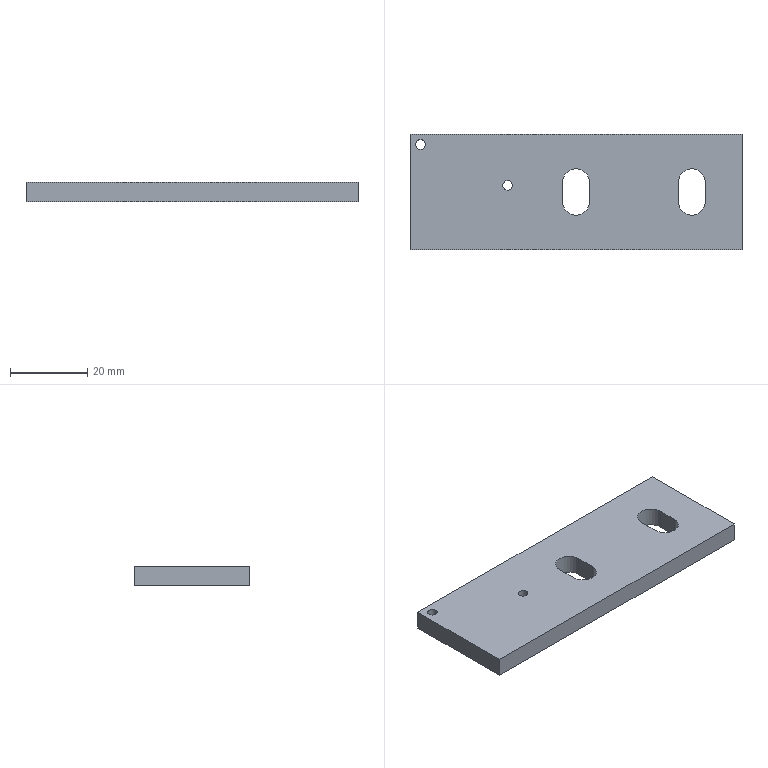Part | STEP file | Square proximity switch plate | 1 solid | 18 faces | box 86 x 30 x 5 mm | volume 12116 mm3 | plane 10 | cylinder 8 | commonest cylinder face diameters 2.5 x4 7 x4
STEP:
#1=CARTESIAN_POINT('',(0.,0.,0.));
#2=DIRECTION('',(0.,0.,1.));
#3=DIRECTION('',(1.,0.,0.));
#4=AXIS2_PLACEMENT_3D('',#1,#2,#3);
#5=CARTESIAN_POINT('',(-16.45,1.7,0.));
#6=VERTEX_POINT('',#5);
#7=CARTESIAN_POINT('',(-16.45,1.7,5.));
#8=VERTEX_POINT('',#7);
#9=CARTESIAN_POINT('',(-16.45,1.7,5.));
#10=DIRECTION('',(0.,0.,1.));
#11=VECTOR('',#10,1.);
#12=LINE('',#9,#11);
#13=CARTESIAN_POINT('',(-17.7,1.7,5.));
#14=DIRECTION('',(0.,0.,1.));
#15=DIRECTION('',(1.,0.,0.));
#16=AXIS2_PLACEMENT_3D('',#13,#14,#15);
#17=CYLINDRICAL_SURFACE('',#16,1.25);
#18=CARTESIAN_POINT('',(6.283,0.));
#19=DIRECTION('',(0.,1.));
#20=VECTOR('',#19,1.);
#21=LINE('',#18,#20);
#22=(GEOMETRIC_REPRESENTATION_CONTEXT(2)PARAMETRIC_REPRESENTATION_CONTEXT()REPRESENTATION_CONTEXT('',''));
#23=DEFINITIONAL_REPRESENTATION('',(#21),#22);
#24=PCURVE('',#17,#23);
#25=CARTESIAN_POINT('',(-17.7,1.7,5.));
#26=DIRECTION('',(0.,0.,1.));
#27=DIRECTION('',(1.,0.,0.));
#28=AXIS2_PLACEMENT_3D('',#25,#26,#27);
#29=CYLINDRICAL_SURFACE('',#28,1.25);
#30=CARTESIAN_POINT('',(0.,0.));
#31=DIRECTION('',(0.,1.));
#32=VECTOR('',#31,1.);
#33=LINE('',#30,#32);
#34=(GEOMETRIC_REPRESENTATION_CONTEXT(2)PARAMETRIC_REPRESENTATION_CONTEXT()REPRESENTATION_CONTEXT('',''));
#35=DEFINITIONAL_REPRESENTATION('',(#33),#34);
#36=PCURVE('',#29,#35);
#37=SURFACE_CURVE('',#12,(#24,#36),.PCURVE_S1.);
#38=EDGE_CURVE('',#6,#8,#37,.T.);
#39=ORIENTED_EDGE('',*,*,#38,.T.);
#40=CARTESIAN_POINT('',(-18.95,1.7,5.));
#41=VERTEX_POINT('',#40);
#42=CARTESIAN_POINT('',(-17.7,1.7,5.));
#43=DIRECTION('',(0.,0.,1.));
#44=DIRECTION('',(1.,0.,0.));
#45=AXIS2_PLACEMENT_3D('',#42,#43,#44);
#46=CIRCLE('',#45,1.25);
#47=CARTESIAN_POINT('',(0.,0.));
#48=DIRECTION('',(1.,0.));
#49=VECTOR('',#48,1.);
#50=LINE('',#47,#49);
#51=(GEOMETRIC_REPRESENTATION_CONTEXT(2)PARAMETRIC_REPRESENTATION_CONTEXT()REPRESENTATION_CONTEXT('',''));
#52=DEFINITIONAL_REPRESENTATION('',(#50),#51);
#53=PCURVE('',#17,#52);
#54=CARTESIAN_POINT('',(0.,0.,5.));
#55=DIRECTION('',(0.,0.,1.));
#56=DIRECTION('',(1.,0.,0.));
#57=AXIS2_PLACEMENT_3D('',#54,#55,#56);
#58=PLANE('',#57);
#59=CARTESIAN_POINT('',(-17.7,1.7));
#60=DIRECTION('',(1.,0.));
#61=AXIS2_PLACEMENT_2D('',#59,#60);
#62=CIRCLE('',#61,1.25);
#63=(GEOMETRIC_REPRESENTATION_CONTEXT(2)PARAMETRIC_REPRESENTATION_CONTEXT()REPRESENTATION_CONTEXT('',''));
#64=DEFINITIONAL_REPRESENTATION('',(#62),#63);
#65=PCURVE('',#58,#64);
#66=SURFACE_CURVE('',#46,(#53,#65),.PCURVE_S1.);
#67=EDGE_CURVE('',#41,#8,#66,.T.);
#68=ORIENTED_EDGE('',*,*,#67,.F.);
#69=CARTESIAN_POINT('',(-18.95,1.7,0.));
#70=VERTEX_POINT('',#69);
#71=CARTESIAN_POINT('',(-18.95,1.7,5.));
#72=DIRECTION('',(0.,0.,1.));
#73=VECTOR('',#72,1.);
#74=LINE('',#71,#73);
#75=CARTESIAN_POINT('',(3.142,0.));
#76=DIRECTION('',(0.,1.));
#77=VECTOR('',#76,1.);
#78=LINE('',#75,#77);
#79=(GEOMETRIC_REPRESENTATION_CONTEXT(2)PARAMETRIC_REPRESENTATION_CONTEXT()REPRESENTATION_CONTEXT('',''));
#80=DEFINITIONAL_REPRESENTATION('',(#78),#79);
#81=PCURVE('',#17,#80);
#82=CARTESIAN_POINT('',(3.142,0.));
#83=DIRECTION('',(0.,1.));
#84=VECTOR('',#83,1.);
#85=LINE('',#82,#84);
#86=(GEOMETRIC_REPRESENTATION_CONTEXT(2)PARAMETRIC_REPRESENTATION_CONTEXT()REPRESENTATION_CONTEXT('',''));
#87=DEFINITIONAL_REPRESENTATION('',(#85),#86);
#88=PCURVE('',#29,#87);
#89=SURFACE_CURVE('',#74,(#81,#88),.PCURVE_S1.);
#90=EDGE_CURVE('',#70,#41,#89,.T.);
#91=ORIENTED_EDGE('',*,*,#90,.F.);
#92=CARTESIAN_POINT('',(-17.7,1.7,0.));
#93=DIRECTION('',(0.,0.,1.));
#94=DIRECTION('',(1.,0.,0.));
#95=AXIS2_PLACEMENT_3D('',#92,#93,#94);
#96=CIRCLE('',#95,1.25);
#97=CARTESIAN_POINT('',(0.,-5.));
#98=DIRECTION('',(1.,0.));
#99=VECTOR('',#98,1.);
#100=LINE('',#97,#99);
#101=(GEOMETRIC_REPRESENTATION_CONTEXT(2)PARAMETRIC_REPRESENTATION_CONTEXT()REPRESENTATION_CONTEXT('',''));
#102=DEFINITIONAL_REPRESENTATION('',(#100),#101);
#103=PCURVE('',#17,#102);
#104=CARTESIAN_POINT('',(0.,0.,0.));
#105=DIRECTION('',(0.,0.,1.));
#106=DIRECTION('',(1.,0.,0.));
#107=AXIS2_PLACEMENT_3D('',#104,#105,#106);
#108=PLANE('',#107);
#109=CARTESIAN_POINT('',(-17.7,1.7));
#110=DIRECTION('',(1.,0.));
#111=AXIS2_PLACEMENT_2D('',#109,#110);
#112=CIRCLE('',#111,1.25);
#113=(GEOMETRIC_REPRESENTATION_CONTEXT(2)PARAMETRIC_REPRESENTATION_CONTEXT()REPRESENTATION_CONTEXT('',''));
#114=DEFINITIONAL_REPRESENTATION('',(#112),#113);
#115=PCURVE('',#108,#114);
#116=SURFACE_CURVE('',#96,(#103,#115),.PCURVE_S1.);
#117=EDGE_CURVE('',#70,#6,#116,.T.);
#118=ORIENTED_EDGE('',*,*,#117,.T.);
#119=EDGE_LOOP('',(#39,#68,#91,#118));
#120=FACE_BOUND('',#119,.F.);
#121=ADVANCED_FACE('',(#120),#17,.F.);
#122=CARTESIAN_POINT('',(-39.05,12.3,0.));
#123=VERTEX_POINT('',#122);
#124=CARTESIAN_POINT('',(-39.05,12.3,5.));
#125=VERTEX_POINT('',#124);
#126=CARTESIAN_POINT('',(-39.05,12.3,5.));
#127=DIRECTION('',(0.,0.,1.));
#128=VECTOR('',#127,1.);
#129=LINE('',#126,#128);
#130=CARTESIAN_POINT('',(-40.3,12.3,5.));
#131=DIRECTION('',(0.,0.,1.));
#132=DIRECTION('',(1.,0.,0.));
#133=AXIS2_PLACEMENT_3D('',#130,#131,#132);
#134=CYLINDRICAL_SURFACE('',#133,1.25);
#135=CARTESIAN_POINT('',(6.283,0.));
#136=DIRECTION('',(0.,1.));
#137=VECTOR('',#136,1.);
#138=LINE('',#135,#137);
#139=(GEOMETRIC_REPRESENTATION_CONTEXT(2)PARAMETRIC_REPRESENTATION_CONTEXT()REPRESENTATION_CONTEXT('',''));
#140=DEFINITIONAL_REPRESENTATION('',(#138),#139);
#141=PCURVE('',#134,#140);
#142=CARTESIAN_POINT('',(-40.3,12.3,5.));
#143=DIRECTION('',(0.,0.,1.));
#144=DIRECTION('',(1.,0.,0.));
#145=AXIS2_PLACEMENT_3D('',#142,#143,#144);
#146=CYLINDRICAL_SURFACE('',#145,1.25);
#147=CARTESIAN_POINT('',(0.,0.));
#148=DIRECTION('',(0.,1.));
#149=VECTOR('',#148,1.);
#150=LINE('',#147,#149);
#151=(GEOMETRIC_REPRESENTATION_CONTEXT(2)PARAMETRIC_REPRESENTATION_CONTEXT()REPRESENTATION_CONTEXT('',''));
#152=DEFINITIONAL_REPRESENTATION('',(#150),#151);
#153=PCURVE('',#146,#152);
#154=SURFACE_CURVE('',#129,(#141,#153),.PCURVE_S1.);
#155=EDGE_CURVE('',#123,#125,#154,.T.);
#156=ORIENTED_EDGE('',*,*,#155,.T.);
#157=CARTESIAN_POINT('',(-41.55,12.3,5.));
#158=VERTEX_POINT('',#157);
#159=CARTESIAN_POINT('',(-40.3,12.3,5.));
#160=DIRECTION('',(0.,0.,1.));
#161=DIRECTION('',(1.,0.,0.));
#162=AXIS2_PLACEMENT_3D('',#159,#160,#161);
#163=CIRCLE('',#162,1.25);
#164=CARTESIAN_POINT('',(0.,0.));
#165=DIRECTION('',(1.,0.));
#166=VECTOR('',#165,1.);
#167=LINE('',#164,#166);
#168=(GEOMETRIC_REPRESENTATION_CONTEXT(2)PARAMETRIC_REPRESENTATION_CONTEXT()REPRESENTATION_CONTEXT('',''));
#169=DEFINITIONAL_REPRESENTATION('',(#167),#168);
#170=PCURVE('',#134,#169);
#171=CARTESIAN_POINT('',(-40.3,12.3));
#172=DIRECTION('',(1.,0.));
#173=AXIS2_PLACEMENT_2D('',#171,#172);
#174=CIRCLE('',#173,1.25);
#175=(GEOMETRIC_REPRESENTATION_CONTEXT(2)PARAMETRIC_REPRESENTATION_CONTEXT()REPRESENTATION_CONTEXT('',''));
#176=DEFINITIONAL_REPRESENTATION('',(#174),#175);
#177=PCURVE('',#58,#176);
#178=SURFACE_CURVE('',#163,(#170,#177),.PCURVE_S1.);
#179=EDGE_CURVE('',#158,#125,#178,.T.);
#180=ORIENTED_EDGE('',*,*,#179,.F.);
#181=CARTESIAN_POINT('',(-41.55,12.3,0.));
#182=VERTEX_POINT('',#181);
#183=CARTESIAN_POINT('',(-41.55,12.3,5.));
#184=DIRECTION('',(0.,0.,1.));
#185=VECTOR('',#184,1.);
#186=LINE('',#183,#185);
#187=CARTESIAN_POINT('',(3.142,0.));
#188=DIRECTION('',(0.,1.));
#189=VECTOR('',#188,1.);
#190=LINE('',#187,#189);
#191=(GEOMETRIC_REPRESENTATION_CONTEXT(2)PARAMETRIC_REPRESENTATION_CONTEXT()REPRESENTATION_CONTEXT('',''));
#192=DEFINITIONAL_REPRESENTATION('',(#190),#191);
#193=PCURVE('',#134,#192);
#194=CARTESIAN_POINT('',(3.142,0.));
#195=DIRECTION('',(0.,1.));
#196=VECTOR('',#195,1.);
#197=LINE('',#194,#196);
#198=(GEOMETRIC_REPRESENTATION_CONTEXT(2)PARAMETRIC_REPRESENTATION_CONTEXT()REPRESENTATION_CONTEXT('',''));
#199=DEFINITIONAL_REPRESENTATION('',(#197),#198);
#200=PCURVE('',#146,#199);
#201=SURFACE_CURVE('',#186,(#193,#200),.PCURVE_S1.);
#202=EDGE_CURVE('',#182,#158,#201,.T.);
#203=ORIENTED_EDGE('',*,*,#202,.F.);
#204=CARTESIAN_POINT('',(-40.3,12.3,0.));
#205=DIRECTION('',(0.,0.,1.));
#206=DIRECTION('',(1.,0.,0.));
#207=AXIS2_PLACEMENT_3D('',#204,#205,#206);
#208=CIRCLE('',#207,1.25);
#209=CARTESIAN_POINT('',(0.,-5.));
#210=DIRECTION('',(1.,0.));
#211=VECTOR('',#210,1.);
#212=LINE('',#209,#211);
#213=(GEOMETRIC_REPRESENTATION_CONTEXT(2)PARAMETRIC_REPRESENTATION_CONTEXT()REPRESENTATION_CONTEXT('',''));
#214=DEFINITIONAL_REPRESENTATION('',(#212),#213);
#215=PCURVE('',#134,#214);
#216=CARTESIAN_POINT('',(-40.3,12.3));
#217=DIRECTION('',(1.,0.));
#218=AXIS2_PLACEMENT_2D('',#216,#217);
#219=CIRCLE('',#218,1.25);
#220=(GEOMETRIC_REPRESENTATION_CONTEXT(2)PARAMETRIC_REPRESENTATION_CONTEXT()REPRESENTATION_CONTEXT('',''));
#221=DEFINITIONAL_REPRESENTATION('',(#219),#220);
#222=PCURVE('',#108,#221);
#223=SURFACE_CURVE('',#208,(#215,#222),.PCURVE_S1.);
#224=EDGE_CURVE('',#182,#123,#223,.T.);
#225=ORIENTED_EDGE('',*,*,#224,.T.);
#226=EDGE_LOOP('',(#156,#180,#203,#225));
#227=FACE_BOUND('',#226,.F.);
#228=ADVANCED_FACE('',(#227),#134,.F.);
#229=CARTESIAN_POINT('',(43.,-15.,0.));
#230=VERTEX_POINT('',#229);
#231=CARTESIAN_POINT('',(43.,15.,0.));
#232=VERTEX_POINT('',#231);
#233=CARTESIAN_POINT('',(43.,15.,0.));
#234=DIRECTION('',(0.,1.,0.));
#235=VECTOR('',#234,1.);
#236=LINE('',#233,#235);
#237=CARTESIAN_POINT('',(43.,15.,5.));
#238=DIRECTION('',(-1.,0.,0.));
#239=DIRECTION('',(0.,0.,1.));
#240=AXIS2_PLACEMENT_3D('',#237,#238,#239);
#241=PLANE('',#240);
#242=CARTESIAN_POINT('',(-5.,0.));
#243=DIRECTION('',(0.,1.));
#244=VECTOR('',#243,1.);
#245=LINE('',#242,#244);
#246=(GEOMETRIC_REPRESENTATION_CONTEXT(2)PARAMETRIC_REPRESENTATION_CONTEXT()REPRESENTATION_CONTEXT('',''));
#247=DEFINITIONAL_REPRESENTATION('',(#245),#246);
#248=PCURVE('',#241,#247);
#249=CARTESIAN_POINT('',(43.,15.));
#250=DIRECTION('',(0.,1.));
#251=VECTOR('',#250,1.);
#252=LINE('',#249,#251);
#253=(GEOMETRIC_REPRESENTATION_CONTEXT(2)PARAMETRIC_REPRESENTATION_CONTEXT()REPRESENTATION_CONTEXT('',''));
#254=DEFINITIONAL_REPRESENTATION('',(#252),#253);
#255=PCURVE('',#108,#254);
#256=SURFACE_CURVE('',#236,(#248,#255),.PCURVE_S1.);
#257=EDGE_CURVE('',#230,#232,#256,.T.);
#258=ORIENTED_EDGE('',*,*,#257,.T.);
#259=CARTESIAN_POINT('',(43.,15.,5.));
#260=VERTEX_POINT('',#259);
#261=CARTESIAN_POINT('',(43.,15.,5.));
#262=DIRECTION('',(0.,0.,-1.));
#263=VECTOR('',#262,1.);
#264=LINE('',#261,#263);
#265=CARTESIAN_POINT('',(0.,0.));
#266=DIRECTION('',(-1.,0.));
#267=VECTOR('',#266,1.);
#268=LINE('',#265,#267);
#269=(GEOMETRIC_REPRESENTATION_CONTEXT(2)PARAMETRIC_REPRESENTATION_CONTEXT()REPRESENTATION_CONTEXT('',''));
#270=DEFINITIONAL_REPRESENTATION('',(#268),#269);
#271=PCURVE('',#241,#270);
#272=CARTESIAN_POINT('',(-43.,15.,5.));
#273=DIRECTION('',(0.,-1.,0.));
#274=DIRECTION('',(0.,0.,-1.));
#275=AXIS2_PLACEMENT_3D('',#272,#273,#274);
#276=PLANE('',#275);
#277=CARTESIAN_POINT('',(0.,86.));
#278=DIRECTION('',(1.,0.));
#279=VECTOR('',#278,1.);
#280=LINE('',#277,#279);
#281=(GEOMETRIC_REPRESENTATION_CONTEXT(2)PARAMETRIC_REPRESENTATION_CONTEXT()REPRESENTATION_CONTEXT('',''));
#282=DEFINITIONAL_REPRESENTATION('',(#280),#281);
#283=PCURVE('',#276,#282);
#284=SURFACE_CURVE('',#264,(#271,#283),.PCURVE_S1.);
#285=EDGE_CURVE('',#260,#232,#284,.T.);
#286=ORIENTED_EDGE('',*,*,#285,.F.);
#287=CARTESIAN_POINT('',(43.,-15.,5.));
#288=VERTEX_POINT('',#287);
#289=CARTESIAN_POINT('',(43.,15.,5.));
#290=DIRECTION('',(0.,1.,0.));
#291=VECTOR('',#290,1.);
#292=LINE('',#289,#291);
#293=CARTESIAN_POINT('',(0.,0.));
#294=DIRECTION('',(0.,1.));
#295=VECTOR('',#294,1.);
#296=LINE('',#293,#295);
#297=(GEOMETRIC_REPRESENTATION_CONTEXT(2)PARAMETRIC_REPRESENTATION_CONTEXT()REPRESENTATION_CONTEXT('',''));
#298=DEFINITIONAL_REPRESENTATION('',(#296),#297);
#299=PCURVE('',#241,#298);
#300=CARTESIAN_POINT('',(43.,15.));
#301=DIRECTION('',(0.,1.));
#302=VECTOR('',#301,1.);
#303=LINE('',#300,#302);
#304=(GEOMETRIC_REPRESENTATION_CONTEXT(2)PARAMETRIC_REPRESENTATION_CONTEXT()REPRESENTATION_CONTEXT('',''));
#305=DEFINITIONAL_REPRESENTATION('',(#303),#304);
#306=PCURVE('',#58,#305);
#307=SURFACE_CURVE('',#292,(#299,#306),.PCURVE_S1.);
#308=EDGE_CURVE('',#288,#260,#307,.T.);
#309=ORIENTED_EDGE('',*,*,#308,.F.);
#310=CARTESIAN_POINT('',(43.,-15.,5.));
#311=DIRECTION('',(0.,0.,-1.));
#312=VECTOR('',#311,1.);
#313=LINE('',#310,#312);
#314=CARTESIAN_POINT('',(0.,-30.));
#315=DIRECTION('',(-1.,0.));
#316=VECTOR('',#315,1.);
#317=LINE('',#314,#316);
#318=(GEOMETRIC_REPRESENTATION_CONTEXT(2)PARAMETRIC_REPRESENTATION_CONTEXT()REPRESENTATION_CONTEXT('',''));
#319=DEFINITIONAL_REPRESENTATION('',(#317),#318);
#320=PCURVE('',#241,#319);
#321=CARTESIAN_POINT('',(-43.,-15.,5.));
#322=DIRECTION('',(0.,1.,0.));
#323=DIRECTION('',(0.,0.,1.));
#324=AXIS2_PLACEMENT_3D('',#321,#322,#323);
#325=PLANE('',#324);
#326=CARTESIAN_POINT('',(0.,86.));
#327=DIRECTION('',(-1.,0.));
#328=VECTOR('',#327,1.);
#329=LINE('',#326,#328);
#330=(GEOMETRIC_REPRESENTATION_CONTEXT(2)PARAMETRIC_REPRESENTATION_CONTEXT()REPRESENTATION_CONTEXT('',''));
#331=DEFINITIONAL_REPRESENTATION('',(#329),#330);
#332=PCURVE('',#325,#331);
#333=SURFACE_CURVE('',#313,(#320,#332),.PCURVE_S1.);
#334=EDGE_CURVE('',#288,#230,#333,.T.);
#335=ORIENTED_EDGE('',*,*,#334,.T.);
#336=EDGE_LOOP('',(#258,#286,#309,#335));
#337=FACE_BOUND('',#336,.T.);
#338=ADVANCED_FACE('',(#337),#241,.F.);
#339=CARTESIAN_POINT('',(-43.,15.,0.));
#340=VERTEX_POINT('',#339);
#341=CARTESIAN_POINT('',(-43.,15.,0.));
#342=DIRECTION('',(-1.,0.,0.));
#343=VECTOR('',#342,1.);
#344=LINE('',#341,#343);
#345=CARTESIAN_POINT('',(5.,0.));
#346=DIRECTION('',(0.,-1.));
#347=VECTOR('',#346,1.);
#348=LINE('',#345,#347);
#349=(GEOMETRIC_REPRESENTATION_CONTEXT(2)PARAMETRIC_REPRESENTATION_CONTEXT()REPRESENTATION_CONTEXT('',''));
#350=DEFINITIONAL_REPRESENTATION('',(#348),#349);
#351=PCURVE('',#276,#350);
#352=CARTESIAN_POINT('',(-43.,15.));
#353=DIRECTION('',(-1.,0.));
#354=VECTOR('',#353,1.);
#355=LINE('',#352,#354);
#356=(GEOMETRIC_REPRESENTATION_CONTEXT(2)PARAMETRIC_REPRESENTATION_CONTEXT()REPRESENTATION_CONTEXT('',''));
#357=DEFINITIONAL_REPRESENTATION('',(#355),#356);
#358=PCURVE('',#108,#357);
#359=SURFACE_CURVE('',#344,(#351,#358),.PCURVE_S1.);
#360=EDGE_CURVE('',#232,#340,#359,.T.);
#361=ORIENTED_EDGE('',*,*,#360,.T.);
#362=CARTESIAN_POINT('',(-43.,15.,5.));
#363=VERTEX_POINT('',#362);
#364=CARTESIAN_POINT('',(-43.,15.,5.));
#365=DIRECTION('',(0.,0.,-1.));
#366=VECTOR('',#365,1.);
#367=LINE('',#364,#366);
#368=CARTESIAN_POINT('',(0.,0.));
#369=DIRECTION('',(1.,0.));
#370=VECTOR('',#369,1.);
#371=LINE('',#368,#370);
#372=(GEOMETRIC_REPRESENTATION_CONTEXT(2)PARAMETRIC_REPRESENTATION_CONTEXT()REPRESENTATION_CONTEXT('',''));
#373=DEFINITIONAL_REPRESENTATION('',(#371),#372);
#374=PCURVE('',#276,#373);
#375=CARTESIAN_POINT('',(-43.,15.,5.));
#376=DIRECTION('',(1.,0.,0.));
#377=DIRECTION('',(0.,0.,-1.));
#378=AXIS2_PLACEMENT_3D('',#375,#376,#377);
#379=PLANE('',#378);
#380=CARTESIAN_POINT('',(0.,0.));
#381=DIRECTION('',(1.,0.));
#382=VECTOR('',#381,1.);
#383=LINE('',#380,#382);
#384=(GEOMETRIC_REPRESENTATION_CONTEXT(2)PARAMETRIC_REPRESENTATION_CONTEXT()REPRESENTATION_CONTEXT('',''));
#385=DEFINITIONAL_REPRESENTATION('',(#383),#384);
#386=PCURVE('',#379,#385);
#387=SURFACE_CURVE('',#367,(#374,#386),.PCURVE_S1.);
#388=EDGE_CURVE('',#363,#340,#387,.T.);
#389=ORIENTED_EDGE('',*,*,#388,.F.);
#390=CARTESIAN_POINT('',(-43.,15.,5.));
#391=DIRECTION('',(-1.,0.,0.));
#392=VECTOR('',#391,1.);
#393=LINE('',#390,#392);
#394=CARTESIAN_POINT('',(0.,0.));
#395=DIRECTION('',(0.,-1.));
#396=VECTOR('',#395,1.);
#397=LINE('',#394,#396);
#398=(GEOMETRIC_REPRESENTATION_CONTEXT(2)PARAMETRIC_REPRESENTATION_CONTEXT()REPRESENTATION_CONTEXT('',''));
#399=DEFINITIONAL_REPRESENTATION('',(#397),#398);
#400=PCURVE('',#276,#399);
#401=CARTESIAN_POINT('',(-43.,15.));
#402=DIRECTION('',(-1.,0.));
#403=VECTOR('',#402,1.);
#404=LINE('',#401,#403);
#405=(GEOMETRIC_REPRESENTATION_CONTEXT(2)PARAMETRIC_REPRESENTATION_CONTEXT()REPRESENTATION_CONTEXT('',''));
#406=DEFINITIONAL_REPRESENTATION('',(#404),#405);
#407=PCURVE('',#58,#406);
#408=SURFACE_CURVE('',#393,(#400,#407),.PCURVE_S1.);
#409=EDGE_CURVE('',#260,#363,#408,.T.);
#410=ORIENTED_EDGE('',*,*,#409,.F.);
#411=ORIENTED_EDGE('',*,*,#285,.T.);
#412=EDGE_LOOP('',(#361,#389,#410,#411));
#413=FACE_BOUND('',#412,.T.);
#414=ADVANCED_FACE('',(#413),#276,.F.);
#415=CARTESIAN_POINT('',(-43.,-15.,0.));
#416=VERTEX_POINT('',#415);
#417=CARTESIAN_POINT('',(-43.,15.,0.));
#418=DIRECTION('',(0.,-1.,0.));
#419=VECTOR('',#418,1.);
#420=LINE('',#417,#419);
#421=CARTESIAN_POINT('',(5.,0.));
#422=DIRECTION('',(0.,-1.));
#423=VECTOR('',#422,1.);
#424=LINE('',#421,#423);
#425=(GEOMETRIC_REPRESENTATION_CONTEXT(2)PARAMETRIC_REPRESENTATION_CONTEXT()REPRESENTATION_CONTEXT('',''));
#426=DEFINITIONAL_REPRESENTATION('',(#424),#425);
#427=PCURVE('',#379,#426);
#428=CARTESIAN_POINT('',(-43.,15.));
#429=DIRECTION('',(0.,-1.));
#430=VECTOR('',#429,1.);
#431=LINE('',#428,#430);
#432=(GEOMETRIC_REPRESENTATION_CONTEXT(2)PARAMETRIC_REPRESENTATION_CONTEXT()REPRESENTATION_CONTEXT('',''));
#433=DEFINITIONAL_REPRESENTATION('',(#431),#432);
#434=PCURVE('',#108,#433);
#435=SURFACE_CURVE('',#420,(#427,#434),.PCURVE_S1.);
#436=EDGE_CURVE('',#340,#416,#435,.T.);
#437=ORIENTED_EDGE('',*,*,#436,.T.);
#438=CARTESIAN_POINT('',(-43.,-15.,5.));
#439=VERTEX_POINT('',#438);
#440=CARTESIAN_POINT('',(-43.,-15.,5.));
#441=DIRECTION('',(0.,0.,-1.));
#442=VECTOR('',#441,1.);
#443=LINE('',#440,#442);
#444=CARTESIAN_POINT('',(0.,-30.));
#445=DIRECTION('',(1.,0.));
#446=VECTOR('',#445,1.);
#447=LINE('',#444,#446);
#448=(GEOMETRIC_REPRESENTATION_CONTEXT(2)PARAMETRIC_REPRESENTATION_CONTEXT()REPRESENTATION_CONTEXT('',''));
#449=DEFINITIONAL_REPRESENTATION('',(#447),#448);
#450=PCURVE('',#379,#449);
#451=CARTESIAN_POINT('',(0.,0.));
#452=DIRECTION('',(-1.,0.));
#453=VECTOR('',#452,1.);
#454=LINE('',#451,#453);
#455=(GEOMETRIC_REPRESENTATION_CONTEXT(2)PARAMETRIC_REPRESENTATION_CONTEXT()REPRESENTATION_CONTEXT('',''));
#456=DEFINITIONAL_REPRESENTATION('',(#454),#455);
#457=PCURVE('',#325,#456);
#458=SURFACE_CURVE('',#443,(#450,#457),.PCURVE_S1.);
#459=EDGE_CURVE('',#439,#416,#458,.T.);
#460=ORIENTED_EDGE('',*,*,#459,.F.);
#461=CARTESIAN_POINT('',(-43.,15.,5.));
#462=DIRECTION('',(0.,-1.,0.));
#463=VECTOR('',#462,1.);
#464=LINE('',#461,#463);
#465=CARTESIAN_POINT('',(0.,0.));
#466=DIRECTION('',(0.,-1.));
#467=VECTOR('',#466,1.);
#468=LINE('',#465,#467);
#469=(GEOMETRIC_REPRESENTATION_CONTEXT(2)PARAMETRIC_REPRESENTATION_CONTEXT()REPRESENTATION_CONTEXT('',''));
#470=DEFINITIONAL_REPRESENTATION('',(#468),#469);
#471=PCURVE('',#379,#470);
#472=CARTESIAN_POINT('',(-43.,15.));
#473=DIRECTION('',(0.,-1.));
#474=VECTOR('',#473,1.);
#475=LINE('',#472,#474);
#476=(GEOMETRIC_REPRESENTATION_CONTEXT(2)PARAMETRIC_REPRESENTATION_CONTEXT()REPRESENTATION_CONTEXT('',''));
#477=DEFINITIONAL_REPRESENTATION('',(#475),#476);
#478=PCURVE('',#58,#477);
#479=SURFACE_CURVE('',#464,(#471,#478),.PCURVE_S1.);
#480=EDGE_CURVE('',#363,#439,#479,.T.);
#481=ORIENTED_EDGE('',*,*,#480,.F.);
#482=ORIENTED_EDGE('',*,*,#388,.T.);
#483=EDGE_LOOP('',(#437,#460,#481,#482));
#484=FACE_BOUND('',#483,.T.);
#485=ADVANCED_FACE('',(#484),#379,.F.);
#486=CARTESIAN_POINT('',(-43.,-15.,0.));
#487=DIRECTION('',(1.,0.,0.));
#488=VECTOR('',#487,1.);
#489=LINE('',#486,#488);
#490=CARTESIAN_POINT('',(-5.,0.));
#491=DIRECTION('',(0.,1.));
#492=VECTOR('',#491,1.);
#493=LINE('',#490,#492);
#494=(GEOMETRIC_REPRESENTATION_CONTEXT(2)PARAMETRIC_REPRESENTATION_CONTEXT()REPRESENTATION_CONTEXT('',''));
#495=DEFINITIONAL_REPRESENTATION('',(#493),#494);
#496=PCURVE('',#325,#495);
#497=CARTESIAN_POINT('',(-43.,-15.));
#498=DIRECTION('',(1.,0.));
#499=VECTOR('',#498,1.);
#500=LINE('',#497,#499);
#501=(GEOMETRIC_REPRESENTATION_CONTEXT(2)PARAMETRIC_REPRESENTATION_CONTEXT()REPRESENTATION_CONTEXT('',''));
#502=DEFINITIONAL_REPRESENTATION('',(#500),#501);
#503=PCURVE('',#108,#502);
#504=SURFACE_CURVE('',#489,(#496,#503),.PCURVE_S1.);
#505=EDGE_CURVE('',#416,#230,#504,.T.);
#506=ORIENTED_EDGE('',*,*,#505,.T.);
#507=ORIENTED_EDGE('',*,*,#334,.F.);
#508=CARTESIAN_POINT('',(-43.,-15.,5.));
#509=DIRECTION('',(1.,0.,0.));
#510=VECTOR('',#509,1.);
#511=LINE('',#508,#510);
#512=CARTESIAN_POINT('',(0.,0.));
#513=DIRECTION('',(0.,1.));
#514=VECTOR('',#513,1.);
#515=LINE('',#512,#514);
#516=(GEOMETRIC_REPRESENTATION_CONTEXT(2)PARAMETRIC_REPRESENTATION_CONTEXT()REPRESENTATION_CONTEXT('',''));
#517=DEFINITIONAL_REPRESENTATION('',(#515),#516);
#518=PCURVE('',#325,#517);
#519=CARTESIAN_POINT('',(-43.,-15.));
#520=DIRECTION('',(1.,0.));
#521=VECTOR('',#520,1.);
#522=LINE('',#519,#521);
#523=(GEOMETRIC_REPRESENTATION_CONTEXT(2)PARAMETRIC_REPRESENTATION_CONTEXT()REPRESENTATION_CONTEXT('',''));
#524=DEFINITIONAL_REPRESENTATION('',(#522),#523);
#525=PCURVE('',#58,#524);
#526=SURFACE_CURVE('',#511,(#518,#525),.PCURVE_S1.);
#527=EDGE_CURVE('',#439,#288,#526,.T.);
#528=ORIENTED_EDGE('',*,*,#527,.F.);
#529=ORIENTED_EDGE('',*,*,#459,.T.);
#530=EDGE_LOOP('',(#506,#507,#528,#529));
#531=FACE_BOUND('',#530,.T.);
#532=ADVANCED_FACE('',(#531),#325,.F.);
#533=CARTESIAN_POINT('',(-17.7,1.7,5.));
#534=DIRECTION('',(0.,0.,1.));
#535=DIRECTION('',(1.,0.,0.));
#536=AXIS2_PLACEMENT_3D('',#533,#534,#535);
#537=CIRCLE('',#536,1.25);
#538=CARTESIAN_POINT('',(-17.7,1.7));
#539=DIRECTION('',(1.,0.));
#540=AXIS2_PLACEMENT_2D('',#538,#539);
#541=CIRCLE('',#540,1.25);
#542=(GEOMETRIC_REPRESENTATION_CONTEXT(2)PARAMETRIC_REPRESENTATION_CONTEXT()REPRESENTATION_CONTEXT('',''));
#543=DEFINITIONAL_REPRESENTATION('',(#541),#542);
#544=PCURVE('',#58,#543);
#545=CARTESIAN_POINT('',(0.,0.));
#546=DIRECTION('',(1.,0.));
#547=VECTOR('',#546,1.);
#548=LINE('',#545,#547);
#549=(GEOMETRIC_REPRESENTATION_CONTEXT(2)PARAMETRIC_REPRESENTATION_CONTEXT()REPRESENTATION_CONTEXT('',''));
#550=DEFINITIONAL_REPRESENTATION('',(#548),#549);
#551=PCURVE('',#29,#550);
#552=SURFACE_CURVE('',#537,(#544,#551),.PCURVE_S1.);
#553=EDGE_CURVE('',#8,#41,#552,.T.);
#554=ORIENTED_EDGE('',*,*,#553,.F.);
#555=ORIENTED_EDGE('',*,*,#67,.F.);
#556=EDGE_LOOP('',(#554,#555));
#557=FACE_BOUND('',#556,.T.);
#558=CARTESIAN_POINT('',(-40.3,12.3,5.));
#559=DIRECTION('',(0.,0.,1.));
#560=DIRECTION('',(1.,0.,0.));
#561=AXIS2_PLACEMENT_3D('',#558,#559,#560);
#562=CIRCLE('',#561,1.25);
#563=CARTESIAN_POINT('',(-40.3,12.3));
#564=DIRECTION('',(1.,0.));
#565=AXIS2_PLACEMENT_2D('',#563,#564);
#566=CIRCLE('',#565,1.25);
#567=(GEOMETRIC_REPRESENTATION_CONTEXT(2)PARAMETRIC_REPRESENTATION_CONTEXT()REPRESENTATION_CONTEXT('',''));
#568=DEFINITIONAL_REPRESENTATION('',(#566),#567);
#569=PCURVE('',#58,#568);
#570=CARTESIAN_POINT('',(0.,0.));
#571=DIRECTION('',(1.,0.));
#572=VECTOR('',#571,1.);
#573=LINE('',#570,#572);
#574=(GEOMETRIC_REPRESENTATION_CONTEXT(2)PARAMETRIC_REPRESENTATION_CONTEXT()REPRESENTATION_CONTEXT('',''));
#575=DEFINITIONAL_REPRESENTATION('',(#573),#574);
#576=PCURVE('',#146,#575);
#577=SURFACE_CURVE('',#562,(#569,#576),.PCURVE_S1.);
#578=EDGE_CURVE('',#125,#158,#577,.T.);
#579=ORIENTED_EDGE('',*,*,#578,.F.);
#580=ORIENTED_EDGE('',*,*,#179,.F.);
#581=EDGE_LOOP('',(#579,#580));
#582=FACE_BOUND('',#581,.T.);
#583=CARTESIAN_POINT('',(3.5,2.5,5.));
#584=VERTEX_POINT('',#583);
#585=CARTESIAN_POINT('',(-3.5,2.5,5.));
#586=VERTEX_POINT('',#585);
#587=CARTESIAN_POINT('',(0.,2.5,5.));
#588=DIRECTION('',(0.,0.,1.));
#589=DIRECTION('',(1.,0.,0.));
#590=AXIS2_PLACEMENT_3D('',#587,#588,#589);
#591=CIRCLE('',#590,3.5);
#592=CARTESIAN_POINT('',(0.,2.5));
#593=DIRECTION('',(1.,0.));
#594=AXIS2_PLACEMENT_2D('',#592,#593);
#595=CIRCLE('',#594,3.5);
#596=(GEOMETRIC_REPRESENTATION_CONTEXT(2)PARAMETRIC_REPRESENTATION_CONTEXT()REPRESENTATION_CONTEXT('',''));
#597=DEFINITIONAL_REPRESENTATION('',(#595),#596);
#598=PCURVE('',#58,#597);
#599=CARTESIAN_POINT('',(0.,2.5,0.));
#600=DIRECTION('',(0.,0.,1.));
#601=DIRECTION('',(1.,0.,0.));
#602=AXIS2_PLACEMENT_3D('',#599,#600,#601);
#603=CYLINDRICAL_SURFACE('',#602,3.5);
#604=CARTESIAN_POINT('',(0.,5.));
#605=DIRECTION('',(1.,0.));
#606=VECTOR('',#605,1.);
#607=LINE('',#604,#606);
#608=(GEOMETRIC_REPRESENTATION_CONTEXT(2)PARAMETRIC_REPRESENTATION_CONTEXT()REPRESENTATION_CONTEXT('',''));
#609=DEFINITIONAL_REPRESENTATION('',(#607),#608);
#610=PCURVE('',#603,#609);
#611=SURFACE_CURVE('',#591,(#598,#610),.PCURVE_S1.);
#612=EDGE_CURVE('',#584,#586,#611,.T.);
#613=ORIENTED_EDGE('',*,*,#612,.F.);
#614=CARTESIAN_POINT('',(3.5,-2.5,5.));
#615=VERTEX_POINT('',#614);
#616=CARTESIAN_POINT('',(3.5,2.5,5.));
#617=DIRECTION('',(0.,1.,0.));
#618=VECTOR('',#617,1.);
#619=LINE('',#616,#618);
#620=CARTESIAN_POINT('',(3.5,2.5));
#621=DIRECTION('',(0.,1.));
#622=VECTOR('',#621,1.);
#623=LINE('',#620,#622);
#624=(GEOMETRIC_REPRESENTATION_CONTEXT(2)PARAMETRIC_REPRESENTATION_CONTEXT()REPRESENTATION_CONTEXT('',''));
#625=DEFINITIONAL_REPRESENTATION('',(#623),#624);
#626=PCURVE('',#58,#625);
#627=CARTESIAN_POINT('',(3.5,2.5,0.));
#628=DIRECTION('',(1.,0.,0.));
#629=DIRECTION('',(0.,1.,0.));
#630=AXIS2_PLACEMENT_3D('',#627,#628,#629);
#631=PLANE('',#630);
#632=CARTESIAN_POINT('',(0.,5.));
#633=DIRECTION('',(1.,0.));
#634=VECTOR('',#633,1.);
#635=LINE('',#632,#634);
#636=(GEOMETRIC_REPRESENTATION_CONTEXT(2)PARAMETRIC_REPRESENTATION_CONTEXT()REPRESENTATION_CONTEXT('',''));
#637=DEFINITIONAL_REPRESENTATION('',(#635),#636);
#638=PCURVE('',#631,#637);
#639=SURFACE_CURVE('',#619,(#626,#638),.PCURVE_S1.);
#640=EDGE_CURVE('',#615,#584,#639,.T.);
#641=ORIENTED_EDGE('',*,*,#640,.F.);
#642=CARTESIAN_POINT('',(-3.5,-2.5,5.));
#643=VERTEX_POINT('',#642);
#644=CARTESIAN_POINT('',(0.,-2.5,5.));
#645=DIRECTION('',(0.,0.,1.));
#646=DIRECTION('',(1.,0.,0.));
#647=AXIS2_PLACEMENT_3D('',#644,#645,#646);
#648=CIRCLE('',#647,3.5);
#649=CARTESIAN_POINT('',(0.,-2.5));
#650=DIRECTION('',(1.,0.));
#651=AXIS2_PLACEMENT_2D('',#649,#650);
#652=CIRCLE('',#651,3.5);
#653=(GEOMETRIC_REPRESENTATION_CONTEXT(2)PARAMETRIC_REPRESENTATION_CONTEXT()REPRESENTATION_CONTEXT('',''));
#654=DEFINITIONAL_REPRESENTATION('',(#652),#653);
#655=PCURVE('',#58,#654);
#656=CARTESIAN_POINT('',(0.,-2.5,0.));
#657=DIRECTION('',(0.,0.,1.));
#658=DIRECTION('',(1.,0.,0.));
#659=AXIS2_PLACEMENT_3D('',#656,#657,#658);
#660=CYLINDRICAL_SURFACE('',#659,3.5);
#661=CARTESIAN_POINT('',(0.,5.));
#662=DIRECTION('',(1.,0.));
#663=VECTOR('',#662,1.);
#664=LINE('',#661,#663);
#665=(GEOMETRIC_REPRESENTATION_CONTEXT(2)PARAMETRIC_REPRESENTATION_CONTEXT()REPRESENTATION_CONTEXT('',''));
#666=DEFINITIONAL_REPRESENTATION('',(#664),#665);
#667=PCURVE('',#660,#666);
#668=SURFACE_CURVE('',#648,(#655,#667),.PCURVE_S1.);
#669=EDGE_CURVE('',#643,#615,#668,.T.);
#670=ORIENTED_EDGE('',*,*,#669,.F.);
#671=CARTESIAN_POINT('',(-3.5,2.5,5.));
#672=DIRECTION('',(0.,-1.,0.));
#673=VECTOR('',#672,1.);
#674=LINE('',#671,#673);
#675=CARTESIAN_POINT('',(-3.5,2.5));
#676=DIRECTION('',(0.,-1.));
#677=VECTOR('',#676,1.);
#678=LINE('',#675,#677);
#679=(GEOMETRIC_REPRESENTATION_CONTEXT(2)PARAMETRIC_REPRESENTATION_CONTEXT()REPRESENTATION_CONTEXT('',''));
#680=DEFINITIONAL_REPRESENTATION('',(#678),#679);
#681=PCURVE('',#58,#680);
#682=CARTESIAN_POINT('',(-3.5,2.5,0.));
#683=DIRECTION('',(-1.,0.,0.));
#684=DIRECTION('',(0.,0.,1.));
#685=AXIS2_PLACEMENT_3D('',#682,#683,#684);
#686=PLANE('',#685);
#687=CARTESIAN_POINT('',(5.,0.));
#688=DIRECTION('',(0.,-1.));
#689=VECTOR('',#688,1.);
#690=LINE('',#687,#689);
#691=(GEOMETRIC_REPRESENTATION_CONTEXT(2)PARAMETRIC_REPRESENTATION_CONTEXT()REPRESENTATION_CONTEXT('',''));
#692=DEFINITIONAL_REPRESENTATION('',(#690),#691);
#693=PCURVE('',#686,#692);
#694=SURFACE_CURVE('',#674,(#681,#693),.PCURVE_S1.);
#695=EDGE_CURVE('',#586,#643,#694,.T.);
#696=ORIENTED_EDGE('',*,*,#695,.F.);
#697=EDGE_LOOP('',(#613,#641,#670,#696));
#698=FACE_BOUND('',#697,.T.);
#699=CARTESIAN_POINT('',(33.5,2.5,5.));
#700=VERTEX_POINT('',#699);
#701=CARTESIAN_POINT('',(26.5,2.5,5.));
#702=VERTEX_POINT('',#701);
#703=CARTESIAN_POINT('',(30.,2.5,5.));
#704=DIRECTION('',(0.,0.,1.));
#705=DIRECTION('',(1.,0.,0.));
#706=AXIS2_PLACEMENT_3D('',#703,#704,#705);
#707=CIRCLE('',#706,3.5);
#708=CARTESIAN_POINT('',(30.,2.5));
#709=DIRECTION('',(1.,0.));
#710=AXIS2_PLACEMENT_2D('',#708,#709);
#711=CIRCLE('',#710,3.5);
#712=(GEOMETRIC_REPRESENTATION_CONTEXT(2)PARAMETRIC_REPRESENTATION_CONTEXT()REPRESENTATION_CONTEXT('',''));
#713=DEFINITIONAL_REPRESENTATION('',(#711),#712);
#714=PCURVE('',#58,#713);
#715=CARTESIAN_POINT('',(30.,2.5,0.));
#716=DIRECTION('',(0.,0.,1.));
#717=DIRECTION('',(1.,0.,0.));
#718=AXIS2_PLACEMENT_3D('',#715,#716,#717);
#719=CYLINDRICAL_SURFACE('',#718,3.5);
#720=CARTESIAN_POINT('',(0.,5.));
#721=DIRECTION('',(1.,0.));
#722=VECTOR('',#721,1.);
#723=LINE('',#720,#722);
#724=(GEOMETRIC_REPRESENTATION_CONTEXT(2)PARAMETRIC_REPRESENTATION_CONTEXT()REPRESENTATION_CONTEXT('',''));
#725=DEFINITIONAL_REPRESENTATION('',(#723),#724);
#726=PCURVE('',#719,#725);
#727=SURFACE_CURVE('',#707,(#714,#726),.PCURVE_S1.);
#728=EDGE_CURVE('',#700,#702,#727,.T.);
#729=ORIENTED_EDGE('',*,*,#728,.F.);
#730=CARTESIAN_POINT('',(33.5,-2.5,5.));
#731=VERTEX_POINT('',#730);
#732=CARTESIAN_POINT('',(33.5,2.5,5.));
#733=DIRECTION('',(0.,1.,0.));
#734=VECTOR('',#733,1.);
#735=LINE('',#732,#734);
#736=CARTESIAN_POINT('',(33.5,2.5));
#737=DIRECTION('',(0.,1.));
#738=VECTOR('',#737,1.);
#739=LINE('',#736,#738);
#740=(GEOMETRIC_REPRESENTATION_CONTEXT(2)PARAMETRIC_REPRESENTATION_CONTEXT()REPRESENTATION_CONTEXT('',''));
#741=DEFINITIONAL_REPRESENTATION('',(#739),#740);
#742=PCURVE('',#58,#741);
#743=CARTESIAN_POINT('',(33.5,2.5,0.));
#744=DIRECTION('',(1.,0.,0.));
#745=DIRECTION('',(0.,1.,0.));
#746=AXIS2_PLACEMENT_3D('',#743,#744,#745);
#747=PLANE('',#746);
#748=CARTESIAN_POINT('',(0.,5.));
#749=DIRECTION('',(1.,0.));
#750=VECTOR('',#749,1.);
#751=LINE('',#748,#750);
#752=(GEOMETRIC_REPRESENTATION_CONTEXT(2)PARAMETRIC_REPRESENTATION_CONTEXT()REPRESENTATION_CONTEXT('',''));
#753=DEFINITIONAL_REPRESENTATION('',(#751),#752);
#754=PCURVE('',#747,#753);
#755=SURFACE_CURVE('',#735,(#742,#754),.PCURVE_S1.);
#756=EDGE_CURVE('',#731,#700,#755,.T.);
#757=ORIENTED_EDGE('',*,*,#756,.F.);
#758=CARTESIAN_POINT('',(26.5,-2.5,5.));
#759=VERTEX_POINT('',#758);
#760=CARTESIAN_POINT('',(30.,-2.5,5.));
#761=DIRECTION('',(0.,0.,1.));
#762=DIRECTION('',(1.,0.,0.));
#763=AXIS2_PLACEMENT_3D('',#760,#761,#762);
#764=CIRCLE('',#763,3.5);
#765=CARTESIAN_POINT('',(30.,-2.5));
#766=DIRECTION('',(1.,0.));
#767=AXIS2_PLACEMENT_2D('',#765,#766);
#768=CIRCLE('',#767,3.5);
#769=(GEOMETRIC_REPRESENTATION_CONTEXT(2)PARAMETRIC_REPRESENTATION_CONTEXT()REPRESENTATION_CONTEXT('',''));
#770=DEFINITIONAL_REPRESENTATION('',(#768),#769);
#771=PCURVE('',#58,#770);
#772=CARTESIAN_POINT('',(30.,-2.5,0.));
#773=DIRECTION('',(0.,0.,1.));
#774=DIRECTION('',(1.,0.,0.));
#775=AXIS2_PLACEMENT_3D('',#772,#773,#774);
#776=CYLINDRICAL_SURFACE('',#775,3.5);
#777=CARTESIAN_POINT('',(0.,5.));
#778=DIRECTION('',(1.,0.));
#779=VECTOR('',#778,1.);
#780=LINE('',#777,#779);
#781=(GEOMETRIC_REPRESENTATION_CONTEXT(2)PARAMETRIC_REPRESENTATION_CONTEXT()REPRESENTATION_CONTEXT('',''));
#782=DEFINITIONAL_REPRESENTATION('',(#780),#781);
#783=PCURVE('',#776,#782);
#784=SURFACE_CURVE('',#764,(#771,#783),.PCURVE_S1.);
#785=EDGE_CURVE('',#759,#731,#784,.T.);
#786=ORIENTED_EDGE('',*,*,#785,.F.);
#787=CARTESIAN_POINT('',(26.5,2.5,5.));
#788=DIRECTION('',(0.,-1.,0.));
#789=VECTOR('',#788,1.);
#790=LINE('',#787,#789);
#791=CARTESIAN_POINT('',(26.5,2.5));
#792=DIRECTION('',(0.,-1.));
#793=VECTOR('',#792,1.);
#794=LINE('',#791,#793);
#795=(GEOMETRIC_REPRESENTATION_CONTEXT(2)PARAMETRIC_REPRESENTATION_CONTEXT()REPRESENTATION_CONTEXT('',''));
#796=DEFINITIONAL_REPRESENTATION('',(#794),#795);
#797=PCURVE('',#58,#796);
#798=CARTESIAN_POINT('',(26.5,2.5,0.));
#799=DIRECTION('',(-1.,0.,0.));
#800=DIRECTION('',(0.,0.,1.));
#801=AXIS2_PLACEMENT_3D('',#798,#799,#800);
#802=PLANE('',#801);
#803=CARTESIAN_POINT('',(5.,0.));
#804=DIRECTION('',(0.,-1.));
#805=VECTOR('',#804,1.);
#806=LINE('',#803,#805);
#807=(GEOMETRIC_REPRESENTATION_CONTEXT(2)PARAMETRIC_REPRESENTATION_CONTEXT()REPRESENTATION_CONTEXT('',''));
#808=DEFINITIONAL_REPRESENTATION('',(#806),#807);
#809=PCURVE('',#802,#808);
#810=SURFACE_CURVE('',#790,(#797,#809),.PCURVE_S1.);
#811=EDGE_CURVE('',#702,#759,#810,.T.);
#812=ORIENTED_EDGE('',*,*,#811,.F.);
#813=EDGE_LOOP('',(#729,#757,#786,#812));
#814=FACE_BOUND('',#813,.T.);
#815=ORIENTED_EDGE('',*,*,#308,.T.);
#816=ORIENTED_EDGE('',*,*,#409,.T.);
#817=ORIENTED_EDGE('',*,*,#480,.T.);
#818=ORIENTED_EDGE('',*,*,#527,.T.);
#819=EDGE_LOOP('',(#815,#816,#817,#818));
#820=FACE_BOUND('',#819,.T.);
#821=ADVANCED_FACE('',(#557,#582,#698,#814,#820),#58,.T.);
#822=CARTESIAN_POINT('',(-17.7,1.7,0.));
#823=DIRECTION('',(0.,0.,1.));
#824=DIRECTION('',(1.,0.,0.));
#825=AXIS2_PLACEMENT_3D('',#822,#823,#824);
#826=CIRCLE('',#825,1.25);
#827=CARTESIAN_POINT('',(-17.7,1.7));
#828=DIRECTION('',(1.,0.));
#829=AXIS2_PLACEMENT_2D('',#827,#828);
#830=CIRCLE('',#829,1.25);
#831=(GEOMETRIC_REPRESENTATION_CONTEXT(2)PARAMETRIC_REPRESENTATION_CONTEXT()REPRESENTATION_CONTEXT('',''));
#832=DEFINITIONAL_REPRESENTATION('',(#830),#831);
#833=PCURVE('',#108,#832);
#834=CARTESIAN_POINT('',(0.,-5.));
#835=DIRECTION('',(1.,0.));
#836=VECTOR('',#835,1.);
#837=LINE('',#834,#836);
#838=(GEOMETRIC_REPRESENTATION_CONTEXT(2)PARAMETRIC_REPRESENTATION_CONTEXT()REPRESENTATION_CONTEXT('',''));
#839=DEFINITIONAL_REPRESENTATION('',(#837),#838);
#840=PCURVE('',#29,#839);
#841=SURFACE_CURVE('',#826,(#833,#840),.PCURVE_S1.);
#842=EDGE_CURVE('',#6,#70,#841,.T.);
#843=ORIENTED_EDGE('',*,*,#842,.T.);
#844=ORIENTED_EDGE('',*,*,#117,.T.);
#845=EDGE_LOOP('',(#843,#844));
#846=FACE_BOUND('',#845,.T.);
#847=CARTESIAN_POINT('',(-40.3,12.3,0.));
#848=DIRECTION('',(0.,0.,1.));
#849=DIRECTION('',(1.,0.,0.));
#850=AXIS2_PLACEMENT_3D('',#847,#848,#849);
#851=CIRCLE('',#850,1.25);
#852=CARTESIAN_POINT('',(-40.3,12.3));
#853=DIRECTION('',(1.,0.));
#854=AXIS2_PLACEMENT_2D('',#852,#853);
#855=CIRCLE('',#854,1.25);
#856=(GEOMETRIC_REPRESENTATION_CONTEXT(2)PARAMETRIC_REPRESENTATION_CONTEXT()REPRESENTATION_CONTEXT('',''));
#857=DEFINITIONAL_REPRESENTATION('',(#855),#856);
#858=PCURVE('',#108,#857);
#859=CARTESIAN_POINT('',(0.,-5.));
#860=DIRECTION('',(1.,0.));
#861=VECTOR('',#860,1.);
#862=LINE('',#859,#861);
#863=(GEOMETRIC_REPRESENTATION_CONTEXT(2)PARAMETRIC_REPRESENTATION_CONTEXT()REPRESENTATION_CONTEXT('',''));
#864=DEFINITIONAL_REPRESENTATION('',(#862),#863);
#865=PCURVE('',#146,#864);
#866=SURFACE_CURVE('',#851,(#858,#865),.PCURVE_S1.);
#867=EDGE_CURVE('',#123,#182,#866,.T.);
#868=ORIENTED_EDGE('',*,*,#867,.T.);
#869=ORIENTED_EDGE('',*,*,#224,.T.);
#870=EDGE_LOOP('',(#868,#869));
#871=FACE_BOUND('',#870,.T.);
#872=CARTESIAN_POINT('',(3.5,-2.5,0.));
#873=VERTEX_POINT('',#872);
#874=CARTESIAN_POINT('',(3.5,2.5,0.));
#875=VERTEX_POINT('',#874);
#876=CARTESIAN_POINT('',(3.5,2.5,0.));
#877=DIRECTION('',(0.,1.,0.));
#878=VECTOR('',#877,1.);
#879=LINE('',#876,#878);
#880=CARTESIAN_POINT('',(3.5,2.5));
#881=DIRECTION('',(0.,1.));
#882=VECTOR('',#881,1.);
#883=LINE('',#880,#882);
#884=(GEOMETRIC_REPRESENTATION_CONTEXT(2)PARAMETRIC_REPRESENTATION_CONTEXT()REPRESENTATION_CONTEXT('',''));
#885=DEFINITIONAL_REPRESENTATION('',(#883),#884);
#886=PCURVE('',#108,#885);
#887=CARTESIAN_POINT('',(0.,0.));
#888=DIRECTION('',(1.,0.));
#889=VECTOR('',#888,1.);
#890=LINE('',#887,#889);
#891=(GEOMETRIC_REPRESENTATION_CONTEXT(2)PARAMETRIC_REPRESENTATION_CONTEXT()REPRESENTATION_CONTEXT('',''));
#892=DEFINITIONAL_REPRESENTATION('',(#890),#891);
#893=PCURVE('',#631,#892);
#894=SURFACE_CURVE('',#879,(#886,#893),.PCURVE_S1.);
#895=EDGE_CURVE('',#873,#875,#894,.T.);
#896=ORIENTED_EDGE('',*,*,#895,.T.);
#897=CARTESIAN_POINT('',(-3.5,2.5,0.));
#898=VERTEX_POINT('',#897);
#899=CARTESIAN_POINT('',(0.,2.5,0.));
#900=DIRECTION('',(0.,0.,1.));
#901=DIRECTION('',(1.,0.,0.));
#902=AXIS2_PLACEMENT_3D('',#899,#900,#901);
#903=CIRCLE('',#902,3.5);
#904=CARTESIAN_POINT('',(0.,2.5));
#905=DIRECTION('',(1.,0.));
#906=AXIS2_PLACEMENT_2D('',#904,#905);
#907=CIRCLE('',#906,3.5);
#908=(GEOMETRIC_REPRESENTATION_CONTEXT(2)PARAMETRIC_REPRESENTATION_CONTEXT()REPRESENTATION_CONTEXT('',''));
#909=DEFINITIONAL_REPRESENTATION('',(#907),#908);
#910=PCURVE('',#108,#909);
#911=CARTESIAN_POINT('',(0.,0.));
#912=DIRECTION('',(1.,0.));
#913=VECTOR('',#912,1.);
#914=LINE('',#911,#913);
#915=(GEOMETRIC_REPRESENTATION_CONTEXT(2)PARAMETRIC_REPRESENTATION_CONTEXT()REPRESENTATION_CONTEXT('',''));
#916=DEFINITIONAL_REPRESENTATION('',(#914),#915);
#917=PCURVE('',#603,#916);
#918=SURFACE_CURVE('',#903,(#910,#917),.PCURVE_S1.);
#919=EDGE_CURVE('',#875,#898,#918,.T.);
#920=ORIENTED_EDGE('',*,*,#919,.T.);
#921=CARTESIAN_POINT('',(-3.5,-2.5,0.));
#922=VERTEX_POINT('',#921);
#923=CARTESIAN_POINT('',(-3.5,2.5,0.));
#924=DIRECTION('',(0.,-1.,0.));
#925=VECTOR('',#924,1.);
#926=LINE('',#923,#925);
#927=CARTESIAN_POINT('',(-3.5,2.5));
#928=DIRECTION('',(0.,-1.));
#929=VECTOR('',#928,1.);
#930=LINE('',#927,#929);
#931=(GEOMETRIC_REPRESENTATION_CONTEXT(2)PARAMETRIC_REPRESENTATION_CONTEXT()REPRESENTATION_CONTEXT('',''));
#932=DEFINITIONAL_REPRESENTATION('',(#930),#931);
#933=PCURVE('',#108,#932);
#934=CARTESIAN_POINT('',(0.,0.));
#935=DIRECTION('',(0.,-1.));
#936=VECTOR('',#935,1.);
#937=LINE('',#934,#936);
#938=(GEOMETRIC_REPRESENTATION_CONTEXT(2)PARAMETRIC_REPRESENTATION_CONTEXT()REPRESENTATION_CONTEXT('',''));
#939=DEFINITIONAL_REPRESENTATION('',(#937),#938);
#940=PCURVE('',#686,#939);
#941=SURFACE_CURVE('',#926,(#933,#940),.PCURVE_S1.);
#942=EDGE_CURVE('',#898,#922,#941,.T.);
#943=ORIENTED_EDGE('',*,*,#942,.T.);
#944=CARTESIAN_POINT('',(0.,-2.5,0.));
#945=DIRECTION('',(0.,0.,1.));
#946=DIRECTION('',(1.,0.,0.));
#947=AXIS2_PLACEMENT_3D('',#944,#945,#946);
#948=CIRCLE('',#947,3.5);
#949=CARTESIAN_POINT('',(0.,-2.5));
#950=DIRECTION('',(1.,0.));
#951=AXIS2_PLACEMENT_2D('',#949,#950);
#952=CIRCLE('',#951,3.5);
#953=(GEOMETRIC_REPRESENTATION_CONTEXT(2)PARAMETRIC_REPRESENTATION_CONTEXT()REPRESENTATION_CONTEXT('',''));
#954=DEFINITIONAL_REPRESENTATION('',(#952),#953);
#955=PCURVE('',#108,#954);
#956=CARTESIAN_POINT('',(0.,0.));
#957=DIRECTION('',(1.,0.));
#958=VECTOR('',#957,1.);
#959=LINE('',#956,#958);
#960=(GEOMETRIC_REPRESENTATION_CONTEXT(2)PARAMETRIC_REPRESENTATION_CONTEXT()REPRESENTATION_CONTEXT('',''));
#961=DEFINITIONAL_REPRESENTATION('',(#959),#960);
#962=PCURVE('',#660,#961);
#963=SURFACE_CURVE('',#948,(#955,#962),.PCURVE_S1.);
#964=EDGE_CURVE('',#922,#873,#963,.T.);
#965=ORIENTED_EDGE('',*,*,#964,.T.);
#966=EDGE_LOOP('',(#896,#920,#943,#965));
#967=FACE_BOUND('',#966,.T.);
#968=CARTESIAN_POINT('',(33.5,-2.5,0.));
#969=VERTEX_POINT('',#968);
#970=CARTESIAN_POINT('',(33.5,2.5,0.));
#971=VERTEX_POINT('',#970);
#972=CARTESIAN_POINT('',(33.5,2.5,0.));
#973=DIRECTION('',(0.,1.,0.));
#974=VECTOR('',#973,1.);
#975=LINE('',#972,#974);
#976=CARTESIAN_POINT('',(33.5,2.5));
#977=DIRECTION('',(0.,1.));
#978=VECTOR('',#977,1.);
#979=LINE('',#976,#978);
#980=(GEOMETRIC_REPRESENTATION_CONTEXT(2)PARAMETRIC_REPRESENTATION_CONTEXT()REPRESENTATION_CONTEXT('',''));
#981=DEFINITIONAL_REPRESENTATION('',(#979),#980);
#982=PCURVE('',#108,#981);
#983=CARTESIAN_POINT('',(0.,0.));
#984=DIRECTION('',(1.,0.));
#985=VECTOR('',#984,1.);
#986=LINE('',#983,#985);
#987=(GEOMETRIC_REPRESENTATION_CONTEXT(2)PARAMETRIC_REPRESENTATION_CONTEXT()REPRESENTATION_CONTEXT('',''));
#988=DEFINITIONAL_REPRESENTATION('',(#986),#987);
#989=PCURVE('',#747,#988);
#990=SURFACE_CURVE('',#975,(#982,#989),.PCURVE_S1.);
#991=EDGE_CURVE('',#969,#971,#990,.T.);
#992=ORIENTED_EDGE('',*,*,#991,.T.);
#993=CARTESIAN_POINT('',(26.5,2.5,0.));
#994=VERTEX_POINT('',#993);
#995=CARTESIAN_POINT('',(30.,2.5,0.));
#996=DIRECTION('',(0.,0.,1.));
#997=DIRECTION('',(1.,0.,0.));
#998=AXIS2_PLACEMENT_3D('',#995,#996,#997);
#999=CIRCLE('',#998,3.5);
#1000=CARTESIAN_POINT('',(30.,2.5));
#1001=DIRECTION('',(1.,0.));
#1002=AXIS2_PLACEMENT_2D('',#1000,#1001);
#1003=CIRCLE('',#1002,3.5);
#1004=(GEOMETRIC_REPRESENTATION_CONTEXT(2)PARAMETRIC_REPRESENTATION_CONTEXT()REPRESENTATION_CONTEXT('',''));
#1005=DEFINITIONAL_REPRESENTATION('',(#1003),#1004);
#1006=PCURVE('',#108,#1005);
#1007=CARTESIAN_POINT('',(0.,0.));
#1008=DIRECTION('',(1.,0.));
#1009=VECTOR('',#1008,1.);
#1010=LINE('',#1007,#1009);
#1011=(GEOMETRIC_REPRESENTATION_CONTEXT(2)PARAMETRIC_REPRESENTATION_CONTEXT()REPRESENTATION_CONTEXT('',''));
#1012=DEFINITIONAL_REPRESENTATION('',(#1010),#1011);
#1013=PCURVE('',#719,#1012);
#1014=SURFACE_CURVE('',#999,(#1006,#1013),.PCURVE_S1.);
#1015=EDGE_CURVE('',#971,#994,#1014,.T.);
#1016=ORIENTED_EDGE('',*,*,#1015,.T.);
#1017=CARTESIAN_POINT('',(26.5,-2.5,0.));
#1018=VERTEX_POINT('',#1017);
#1019=CARTESIAN_POINT('',(26.5,2.5,0.));
#1020=DIRECTION('',(0.,-1.,0.));
#1021=VECTOR('',#1020,1.);
#1022=LINE('',#1019,#1021);
#1023=CARTESIAN_POINT('',(26.5,2.5));
#1024=DIRECTION('',(0.,-1.));
#1025=VECTOR('',#1024,1.);
#1026=LINE('',#1023,#1025);
#1027=(GEOMETRIC_REPRESENTATION_CONTEXT(2)PARAMETRIC_REPRESENTATION_CONTEXT()REPRESENTATION_CONTEXT('',''));
#1028=DEFINITIONAL_REPRESENTATION('',(#1026),#1027);
#1029=PCURVE('',#108,#1028);
#1030=CARTESIAN_POINT('',(0.,0.));
#1031=DIRECTION('',(0.,-1.));
#1032=VECTOR('',#1031,1.);
#1033=LINE('',#1030,#1032);
#1034=(GEOMETRIC_REPRESENTATION_CONTEXT(2)PARAMETRIC_REPRESENTATION_CONTEXT()REPRESENTATION_CONTEXT('',''));
#1035=DEFINITIONAL_REPRESENTATION('',(#1033),#1034);
#1036=PCURVE('',#802,#1035);
#1037=SURFACE_CURVE('',#1022,(#1029,#1036),.PCURVE_S1.);
#1038=EDGE_CURVE('',#994,#1018,#1037,.T.);
#1039=ORIENTED_EDGE('',*,*,#1038,.T.);
#1040=CARTESIAN_POINT('',(30.,-2.5,0.));
#1041=DIRECTION('',(0.,0.,1.));
#1042=DIRECTION('',(1.,0.,0.));
#1043=AXIS2_PLACEMENT_3D('',#1040,#1041,#1042);
#1044=CIRCLE('',#1043,3.5);
#1045=CARTESIAN_POINT('',(30.,-2.5));
#1046=DIRECTION('',(1.,0.));
#1047=AXIS2_PLACEMENT_2D('',#1045,#1046);
#1048=CIRCLE('',#1047,3.5);
#1049=(GEOMETRIC_REPRESENTATION_CONTEXT(2)PARAMETRIC_REPRESENTATION_CONTEXT()REPRESENTATION_CONTEXT('',''));
#1050=DEFINITIONAL_REPRESENTATION('',(#1048),#1049);
#1051=PCURVE('',#108,#1050);
#1052=CARTESIAN_POINT('',(0.,0.));
#1053=DIRECTION('',(1.,0.));
#1054=VECTOR('',#1053,1.);
#1055=LINE('',#1052,#1054);
#1056=(GEOMETRIC_REPRESENTATION_CONTEXT(2)PARAMETRIC_REPRESENTATION_CONTEXT()REPRESENTATION_CONTEXT('',''));
#1057=DEFINITIONAL_REPRESENTATION('',(#1055),#1056);
#1058=PCURVE('',#776,#1057);
#1059=SURFACE_CURVE('',#1044,(#1051,#1058),.PCURVE_S1.);
#1060=EDGE_CURVE('',#1018,#969,#1059,.T.);
#1061=ORIENTED_EDGE('',*,*,#1060,.T.);
#1062=EDGE_LOOP('',(#992,#1016,#1039,#1061));
#1063=FACE_BOUND('',#1062,.T.);
#1064=ORIENTED_EDGE('',*,*,#257,.F.);
#1065=ORIENTED_EDGE('',*,*,#505,.F.);
#1066=ORIENTED_EDGE('',*,*,#436,.F.);
#1067=ORIENTED_EDGE('',*,*,#360,.F.);
#1068=EDGE_LOOP('',(#1064,#1065,#1066,#1067));
#1069=FACE_BOUND('',#1068,.T.);
#1070=ADVANCED_FACE('',(#846,#871,#967,#1063,#1069),#108,.F.);
#1071=CARTESIAN_POINT('',(33.5,2.5,0.));
#1072=DIRECTION('',(0.,0.,1.));
#1073=VECTOR('',#1072,1.);
#1074=LINE('',#1071,#1073);
#1075=CARTESIAN_POINT('',(0.,0.));
#1076=DIRECTION('',(0.,1.));
#1077=VECTOR('',#1076,1.);
#1078=LINE('',#1075,#1077);
#1079=(GEOMETRIC_REPRESENTATION_CONTEXT(2)PARAMETRIC_REPRESENTATION_CONTEXT()REPRESENTATION_CONTEXT('',''));
#1080=DEFINITIONAL_REPRESENTATION('',(#1078),#1079);
#1081=PCURVE('',#719,#1080);
#1082=CARTESIAN_POINT('',(0.,0.));
#1083=DIRECTION('',(0.,1.));
#1084=VECTOR('',#1083,1.);
#1085=LINE('',#1082,#1084);
#1086=(GEOMETRIC_REPRESENTATION_CONTEXT(2)PARAMETRIC_REPRESENTATION_CONTEXT()REPRESENTATION_CONTEXT('',''));
#1087=DEFINITIONAL_REPRESENTATION('',(#1085),#1086);
#1088=PCURVE('',#747,#1087);
#1089=SURFACE_CURVE('',#1074,(#1081,#1088),.PCURVE_S1.);
#1090=EDGE_CURVE('',#971,#700,#1089,.T.);
#1091=ORIENTED_EDGE('',*,*,#1090,.F.);
#1092=ORIENTED_EDGE('',*,*,#1015,.T.);
#1093=CARTESIAN_POINT('',(26.5,2.5,0.));
#1094=DIRECTION('',(0.,0.,1.));
#1095=VECTOR('',#1094,1.);
#1096=LINE('',#1093,#1095);
#1097=CARTESIAN_POINT('',(3.142,0.));
#1098=DIRECTION('',(0.,1.));
#1099=VECTOR('',#1098,1.);
#1100=LINE('',#1097,#1099);
#1101=(GEOMETRIC_REPRESENTATION_CONTEXT(2)PARAMETRIC_REPRESENTATION_CONTEXT()REPRESENTATION_CONTEXT('',''));
#1102=DEFINITIONAL_REPRESENTATION('',(#1100),#1101);
#1103=PCURVE('',#719,#1102);
#1104=CARTESIAN_POINT('',(0.,0.));
#1105=DIRECTION('',(1.,0.));
#1106=VECTOR('',#1105,1.);
#1107=LINE('',#1104,#1106);
#1108=(GEOMETRIC_REPRESENTATION_CONTEXT(2)PARAMETRIC_REPRESENTATION_CONTEXT()REPRESENTATION_CONTEXT('',''));
#1109=DEFINITIONAL_REPRESENTATION('',(#1107),#1108);
#1110=PCURVE('',#802,#1109);
#1111=SURFACE_CURVE('',#1096,(#1103,#1110),.PCURVE_S1.);
#1112=EDGE_CURVE('',#994,#702,#1111,.T.);
#1113=ORIENTED_EDGE('',*,*,#1112,.T.);
#1114=ORIENTED_EDGE('',*,*,#728,.F.);
#1115=EDGE_LOOP('',(#1091,#1092,#1113,#1114));
#1116=FACE_BOUND('',#1115,.F.);
#1117=ADVANCED_FACE('',(#1116),#719,.F.);
#1118=ORIENTED_EDGE('',*,*,#756,.T.);
#1119=ORIENTED_EDGE('',*,*,#1090,.F.);
#1120=ORIENTED_EDGE('',*,*,#991,.F.);
#1121=CARTESIAN_POINT('',(33.5,-2.5,0.));
#1122=DIRECTION('',(0.,0.,1.));
#1123=VECTOR('',#1122,1.);
#1124=LINE('',#1121,#1123);
#1125=CARTESIAN_POINT('',(-5.,0.));
#1126=DIRECTION('',(0.,1.));
#1127=VECTOR('',#1126,1.);
#1128=LINE('',#1125,#1127);
#1129=(GEOMETRIC_REPRESENTATION_CONTEXT(2)PARAMETRIC_REPRESENTATION_CONTEXT()REPRESENTATION_CONTEXT('',''));
#1130=DEFINITIONAL_REPRESENTATION('',(#1128),#1129);
#1131=PCURVE('',#747,#1130);
#1132=CARTESIAN_POINT('',(6.283,0.));
#1133=DIRECTION('',(0.,1.));
#1134=VECTOR('',#1133,1.);
#1135=LINE('',#1132,#1134);
#1136=(GEOMETRIC_REPRESENTATION_CONTEXT(2)PARAMETRIC_REPRESENTATION_CONTEXT()REPRESENTATION_CONTEXT('',''));
#1137=DEFINITIONAL_REPRESENTATION('',(#1135),#1136);
#1138=PCURVE('',#776,#1137);
#1139=SURFACE_CURVE('',#1124,(#1131,#1138),.PCURVE_S1.);
#1140=EDGE_CURVE('',#969,#731,#1139,.T.);
#1141=ORIENTED_EDGE('',*,*,#1140,.T.);
#1142=EDGE_LOOP('',(#1118,#1119,#1120,#1141));
#1143=FACE_BOUND('',#1142,.T.);
#1144=ADVANCED_FACE('',(#1143),#747,.F.);
#1145=CARTESIAN_POINT('',(26.5,-2.5,0.));
#1146=DIRECTION('',(0.,0.,1.));
#1147=VECTOR('',#1146,1.);
#1148=LINE('',#1145,#1147);
#1149=CARTESIAN_POINT('',(3.142,0.));
#1150=DIRECTION('',(0.,1.));
#1151=VECTOR('',#1150,1.);
#1152=LINE('',#1149,#1151);
#1153=(GEOMETRIC_REPRESENTATION_CONTEXT(2)PARAMETRIC_REPRESENTATION_CONTEXT()REPRESENTATION_CONTEXT('',''));
#1154=DEFINITIONAL_REPRESENTATION('',(#1152),#1153);
#1155=PCURVE('',#776,#1154);
#1156=CARTESIAN_POINT('',(0.,-5.));
#1157=DIRECTION('',(1.,0.));
#1158=VECTOR('',#1157,1.);
#1159=LINE('',#1156,#1158);
#1160=(GEOMETRIC_REPRESENTATION_CONTEXT(2)PARAMETRIC_REPRESENTATION_CONTEXT()REPRESENTATION_CONTEXT('',''));
#1161=DEFINITIONAL_REPRESENTATION('',(#1159),#1160);
#1162=PCURVE('',#802,#1161);
#1163=SURFACE_CURVE('',#1148,(#1155,#1162),.PCURVE_S1.);
#1164=EDGE_CURVE('',#1018,#759,#1163,.T.);
#1165=ORIENTED_EDGE('',*,*,#1164,.F.);
#1166=ORIENTED_EDGE('',*,*,#1060,.T.);
#1167=ORIENTED_EDGE('',*,*,#1140,.T.);
#1168=ORIENTED_EDGE('',*,*,#785,.F.);
#1169=EDGE_LOOP('',(#1165,#1166,#1167,#1168));
#1170=FACE_BOUND('',#1169,.F.);
#1171=ADVANCED_FACE('',(#1170),#776,.F.);
#1172=ORIENTED_EDGE('',*,*,#811,.T.);
#1173=ORIENTED_EDGE('',*,*,#1164,.F.);
#1174=ORIENTED_EDGE('',*,*,#1038,.F.);
#1175=ORIENTED_EDGE('',*,*,#1112,.T.);
#1176=EDGE_LOOP('',(#1172,#1173,#1174,#1175));
#1177=FACE_BOUND('',#1176,.T.);
#1178=ADVANCED_FACE('',(#1177),#802,.F.);
#1179=CARTESIAN_POINT('',(3.5,2.5,0.));
#1180=DIRECTION('',(0.,0.,1.));
#1181=VECTOR('',#1180,1.);
#1182=LINE('',#1179,#1181);
#1183=CARTESIAN_POINT('',(0.,0.));
#1184=DIRECTION('',(0.,1.));
#1185=VECTOR('',#1184,1.);
#1186=LINE('',#1183,#1185);
#1187=(GEOMETRIC_REPRESENTATION_CONTEXT(2)PARAMETRIC_REPRESENTATION_CONTEXT()REPRESENTATION_CONTEXT('',''));
#1188=DEFINITIONAL_REPRESENTATION('',(#1186),#1187);
#1189=PCURVE('',#603,#1188);
#1190=CARTESIAN_POINT('',(0.,0.));
#1191=DIRECTION('',(0.,1.));
#1192=VECTOR('',#1191,1.);
#1193=LINE('',#1190,#1192);
#1194=(GEOMETRIC_REPRESENTATION_CONTEXT(2)PARAMETRIC_REPRESENTATION_CONTEXT()REPRESENTATION_CONTEXT('',''));
#1195=DEFINITIONAL_REPRESENTATION('',(#1193),#1194);
#1196=PCURVE('',#631,#1195);
#1197=SURFACE_CURVE('',#1182,(#1189,#1196),.PCURVE_S1.);
#1198=EDGE_CURVE('',#875,#584,#1197,.T.);
#1199=ORIENTED_EDGE('',*,*,#1198,.F.);
#1200=ORIENTED_EDGE('',*,*,#919,.T.);
#1201=CARTESIAN_POINT('',(-3.5,2.5,0.));
#1202=DIRECTION('',(0.,0.,1.));
#1203=VECTOR('',#1202,1.);
#1204=LINE('',#1201,#1203);
#1205=CARTESIAN_POINT('',(3.142,0.));
#1206=DIRECTION('',(0.,1.));
#1207=VECTOR('',#1206,1.);
#1208=LINE('',#1205,#1207);
#1209=(GEOMETRIC_REPRESENTATION_CONTEXT(2)PARAMETRIC_REPRESENTATION_CONTEXT()REPRESENTATION_CONTEXT('',''));
#1210=DEFINITIONAL_REPRESENTATION('',(#1208),#1209);
#1211=PCURVE('',#603,#1210);
#1212=CARTESIAN_POINT('',(0.,0.));
#1213=DIRECTION('',(1.,0.));
#1214=VECTOR('',#1213,1.);
#1215=LINE('',#1212,#1214);
#1216=(GEOMETRIC_REPRESENTATION_CONTEXT(2)PARAMETRIC_REPRESENTATION_CONTEXT()REPRESENTATION_CONTEXT('',''));
#1217=DEFINITIONAL_REPRESENTATION('',(#1215),#1216);
#1218=PCURVE('',#686,#1217);
#1219=SURFACE_CURVE('',#1204,(#1211,#1218),.PCURVE_S1.);
#1220=EDGE_CURVE('',#898,#586,#1219,.T.);
#1221=ORIENTED_EDGE('',*,*,#1220,.T.);
#1222=ORIENTED_EDGE('',*,*,#612,.F.);
#1223=EDGE_LOOP('',(#1199,#1200,#1221,#1222));
#1224=FACE_BOUND('',#1223,.F.);
#1225=ADVANCED_FACE('',(#1224),#603,.F.);
#1226=ORIENTED_EDGE('',*,*,#640,.T.);
#1227=ORIENTED_EDGE('',*,*,#1198,.F.);
#1228=ORIENTED_EDGE('',*,*,#895,.F.);
#1229=CARTESIAN_POINT('',(3.5,-2.5,0.));
#1230=DIRECTION('',(0.,0.,1.));
#1231=VECTOR('',#1230,1.);
#1232=LINE('',#1229,#1231);
#1233=CARTESIAN_POINT('',(-5.,0.));
#1234=DIRECTION('',(0.,1.));
#1235=VECTOR('',#1234,1.);
#1236=LINE('',#1233,#1235);
#1237=(GEOMETRIC_REPRESENTATION_CONTEXT(2)PARAMETRIC_REPRESENTATION_CONTEXT()REPRESENTATION_CONTEXT('',''));
#1238=DEFINITIONAL_REPRESENTATION('',(#1236),#1237);
#1239=PCURVE('',#631,#1238);
#1240=CARTESIAN_POINT('',(6.283,0.));
#1241=DIRECTION('',(0.,1.));
#1242=VECTOR('',#1241,1.);
#1243=LINE('',#1240,#1242);
#1244=(GEOMETRIC_REPRESENTATION_CONTEXT(2)PARAMETRIC_REPRESENTATION_CONTEXT()REPRESENTATION_CONTEXT('',''));
#1245=DEFINITIONAL_REPRESENTATION('',(#1243),#1244);
#1246=PCURVE('',#660,#1245);
#1247=SURFACE_CURVE('',#1232,(#1239,#1246),.PCURVE_S1.);
#1248=EDGE_CURVE('',#873,#615,#1247,.T.);
#1249=ORIENTED_EDGE('',*,*,#1248,.T.);
#1250=EDGE_LOOP('',(#1226,#1227,#1228,#1249));
#1251=FACE_BOUND('',#1250,.T.);
#1252=ADVANCED_FACE('',(#1251),#631,.F.);
#1253=CARTESIAN_POINT('',(-3.5,-2.5,0.));
#1254=DIRECTION('',(0.,0.,1.));
#1255=VECTOR('',#1254,1.);
#1256=LINE('',#1253,#1255);
#1257=CARTESIAN_POINT('',(3.142,0.));
#1258=DIRECTION('',(0.,1.));
#1259=VECTOR('',#1258,1.);
#1260=LINE('',#1257,#1259);
#1261=(GEOMETRIC_REPRESENTATION_CONTEXT(2)PARAMETRIC_REPRESENTATION_CONTEXT()REPRESENTATION_CONTEXT('',''));
#1262=DEFINITIONAL_REPRESENTATION('',(#1260),#1261);
#1263=PCURVE('',#660,#1262);
#1264=CARTESIAN_POINT('',(0.,-5.));
#1265=DIRECTION('',(1.,0.));
#1266=VECTOR('',#1265,1.);
#1267=LINE('',#1264,#1266);
#1268=(GEOMETRIC_REPRESENTATION_CONTEXT(2)PARAMETRIC_REPRESENTATION_CONTEXT()REPRESENTATION_CONTEXT('',''));
#1269=DEFINITIONAL_REPRESENTATION('',(#1267),#1268);
#1270=PCURVE('',#686,#1269);
#1271=SURFACE_CURVE('',#1256,(#1263,#1270),.PCURVE_S1.);
#1272=EDGE_CURVE('',#922,#643,#1271,.T.);
#1273=ORIENTED_EDGE('',*,*,#1272,.F.);
#1274=ORIENTED_EDGE('',*,*,#964,.T.);
#1275=ORIENTED_EDGE('',*,*,#1248,.T.);
#1276=ORIENTED_EDGE('',*,*,#669,.F.);
#1277=EDGE_LOOP('',(#1273,#1274,#1275,#1276));
#1278=FACE_BOUND('',#1277,.F.);
#1279=ADVANCED_FACE('',(#1278),#660,.F.);
#1280=ORIENTED_EDGE('',*,*,#695,.T.);
#1281=ORIENTED_EDGE('',*,*,#1272,.F.);
#1282=ORIENTED_EDGE('',*,*,#942,.F.);
#1283=ORIENTED_EDGE('',*,*,#1220,.T.);
#1284=EDGE_LOOP('',(#1280,#1281,#1282,#1283));
#1285=FACE_BOUND('',#1284,.T.);
#1286=ADVANCED_FACE('',(#1285),#686,.F.);
#1287=ORIENTED_EDGE('',*,*,#578,.F.);
#1288=ORIENTED_EDGE('',*,*,#155,.F.);
#1289=ORIENTED_EDGE('',*,*,#867,.T.);
#1290=ORIENTED_EDGE('',*,*,#202,.T.);
#1291=EDGE_LOOP('',(#1287,#1288,#1289,#1290));
#1292=FACE_BOUND('',#1291,.F.);
#1293=ADVANCED_FACE('',(#1292),#146,.F.);
#1294=ORIENTED_EDGE('',*,*,#553,.F.);
#1295=ORIENTED_EDGE('',*,*,#38,.F.);
#1296=ORIENTED_EDGE('',*,*,#842,.T.);
#1297=ORIENTED_EDGE('',*,*,#90,.T.);
#1298=EDGE_LOOP('',(#1294,#1295,#1296,#1297));
#1299=FACE_BOUND('',#1298,.F.);
#1300=ADVANCED_FACE('',(#1299),#29,.F.);
#1301=CLOSED_SHELL('',(#121,#228,#338,#414,#485,#532,#821,#1070,#1117,#1144,#1171,#1178,#1225,#1252,#1279,#1286,#1293,#1300));
#1302=MANIFOLD_SOLID_BREP('',#1301);
#1303=(LENGTH_UNIT()NAMED_UNIT(*)SI_UNIT(.MILLI.,.METRE.));
#1304=UNCERTAINTY_MEASURE_WITH_UNIT(LENGTH_MEASURE(0.0000001),#1303,'','');
#1305=(NAMED_UNIT(*)PLANE_ANGLE_UNIT()SI_UNIT($,.RADIAN.));
#1306=(NAMED_UNIT(*)SI_UNIT($,.STERADIAN.)SOLID_ANGLE_UNIT());
#1307=(GEOMETRIC_REPRESENTATION_CONTEXT(3)GLOBAL_UNCERTAINTY_ASSIGNED_CONTEXT((#1304))GLOBAL_UNIT_ASSIGNED_CONTEXT((#1303,#1305,#1306))REPRESENTATION_CONTEXT('',''));
#1308=ADVANCED_BREP_SHAPE_REPRESENTATION('',(#4,#1302),#1307);